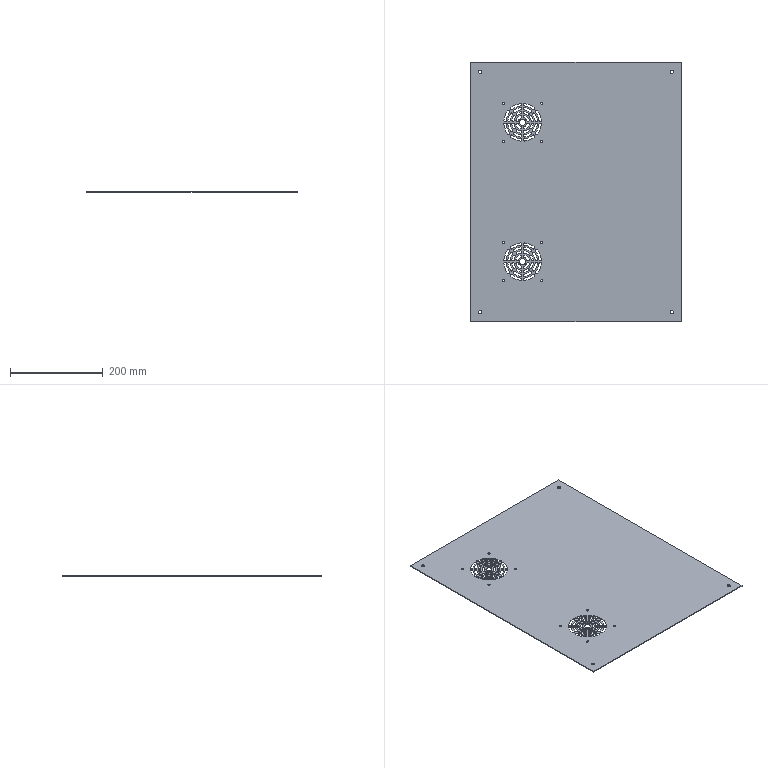Part | STEP file | 09-27 closing plate D (Default) | 1 solid | 314 faces | box 453 x 558 x 1.5 mm | volume 370766 mm3 | cylinder 308 | plane 6 | commonest cylinder face diameters 5 x168 4.5 x16 37 x16 47 x16 54 x16 64 x16